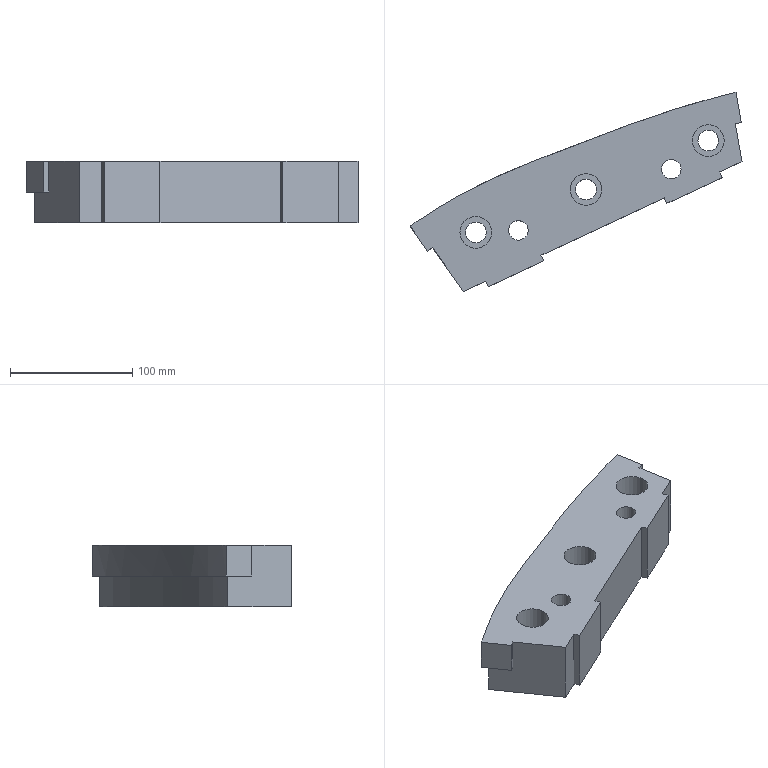Part | NX | features solid 2 | 1 solid | 31 faces | box 271.385 x 162.804 x 50 mm | volume 822513 mm3 | plane 21 | cylinder 8 | spline 2 | commonest cylinder face diameters 17 x3 26 x3 16 x2
STEP:
#1=CARTESIAN_POINT('',(-324.107,502.143,-25.));
#2=VERTEX_POINT('',#1);
#3=CARTESIAN_POINT('',(-319.766,477.523,-25.));
#4=VERTEX_POINT('',#3);
#5=CARTESIAN_POINT('',(-314.512,447.729,-25.));
#6=DIRECTION('',(0.1736,-0.9848,0.));
#7=VECTOR('',#6,1000.);
#8=LINE('',#5,#7);
#9=EDGE_CURVE('',#2,#4,#8,.T.);
#10=ORIENTED_EDGE('',*,*,#9,.T.);
#11=CARTESIAN_POINT('',(-324.69,476.655,-25.));
#12=VERTEX_POINT('',#11);
#13=CARTESIAN_POINT('',(-314.842,478.391,-25.));
#14=DIRECTION('',(-0.9848,-0.1736,0.));
#15=VECTOR('',#14,1000.);
#16=LINE('',#13,#15);
#17=EDGE_CURVE('',#4,#12,#16,.T.);
#18=ORIENTED_EDGE('',*,*,#17,.T.);
#19=CARTESIAN_POINT('',(-328.108,496.039,-25.));
#20=VERTEX_POINT('',#19);
#21=CARTESIAN_POINT('',(-319.436,446.861,-25.));
#22=DIRECTION('',(0.1736,-0.9848,0.));
#23=VECTOR('',#22,1000.);
#24=LINE('',#21,#23);
#25=EDGE_CURVE('',#12,#20,#24,.F.);
#26=ORIENTED_EDGE('',*,*,#25,.T.);
#27=CARTESIAN_POINT('',(-583.566,391.623,-25.));
#28=VERTEX_POINT('',#27);
#29=CARTESIAN_POINT('',(-328.108,496.039,-25.));
#30=CARTESIAN_POINT('',(-339.325,493.302,-25.));
#31=CARTESIAN_POINT('',(-361.624,487.369,-25.));
#32=CARTESIAN_POINT('',(-394.475,476.632,-25.));
#33=CARTESIAN_POINT('',(-427.053,464.52,-25.));
#34=CARTESIAN_POINT('',(-470.494,447.928,-25.));
#35=CARTESIAN_POINT('',(-513.833,431.597,-25.));
#36=CARTESIAN_POINT('',(-554.468,410.285,-25.));
#37=CARTESIAN_POINT('',(-573.98,398.021,-25.));
#38=CARTESIAN_POINT('',(-583.566,391.623,-25.));
#39=B_SPLINE_CURVE_WITH_KNOTS('',3,(#29,#30,#31,#32,#33,#34,#35,#36,#37,#38),.UNSPECIFIED.,.F.,.F.,(4,1,1,1,1,1,1,4),(0.01867,0.1407,0.2627,0.3848,0.5068,0.7508,0.8729,0.9949),.UNSPECIFIED.);
#40=EDGE_CURVE('',#20,#28,#39,.T.);
#41=ORIENTED_EDGE('',*,*,#40,.T.);
#42=CARTESIAN_POINT('',(-572.103,375.253,-25.));
#43=VERTEX_POINT('',#42);
#44=CARTESIAN_POINT('',(-547.462,340.061,-25.));
#45=DIRECTION('',(0.5736,-0.8192,0.));
#46=VECTOR('',#45,1000.);
#47=LINE('',#44,#46);
#48=EDGE_CURVE('',#43,#28,#47,.F.);
#49=ORIENTED_EDGE('',*,*,#48,.F.);
#50=CARTESIAN_POINT('',(-576.199,372.385,-25.));
#51=VERTEX_POINT('',#50);
#52=CARTESIAN_POINT('',(-580.295,369.517,-25.));
#53=DIRECTION('',(0.8192,0.5736,0.));
#54=VECTOR('',#53,1000.);
#55=LINE('',#52,#54);
#56=EDGE_CURVE('',#51,#43,#55,.T.);
#57=ORIENTED_EDGE('',*,*,#56,.F.);
#58=CARTESIAN_POINT('',(-590.588,392.934,-25.));
#59=VERTEX_POINT('',#58);
#60=CARTESIAN_POINT('',(-551.558,337.193,-25.));
#61=DIRECTION('',(0.5736,-0.8192,0.));
#62=VECTOR('',#61,1000.);
#63=LINE('',#60,#62);
#64=EDGE_CURVE('',#59,#51,#63,.T.);
#65=ORIENTED_EDGE('',*,*,#64,.F.);
#66=CARTESIAN_POINT('',(-324.107,502.143,-25.));
#67=CARTESIAN_POINT('',(-341.077,498.12,-25.));
#68=CARTESIAN_POINT('',(-376.687,488.492,-25.));
#69=CARTESIAN_POINT('',(-420.452,472.38,-25.));
#70=CARTESIAN_POINT('',(-456.779,458.517,-25.));
#71=CARTESIAN_POINT('',(-484.05,448.183,-25.));
#72=CARTESIAN_POINT('',(-511.125,437.331,-25.));
#73=CARTESIAN_POINT('',(-546.415,420.942,-25.));
#74=CARTESIAN_POINT('',(-571.409,405.8,-25.));
#75=CARTESIAN_POINT('',(-587.555,394.969,-25.));
#76=CARTESIAN_POINT('',(-595.462,389.665,-25.));
#77=CARTESIAN_POINT('',(-603.368,384.361,-25.));
#78=CARTESIAN_POINT('',(-611.275,379.057,-25.));
#79=B_SPLINE_CURVE_WITH_KNOTS('',3,(#66,#67,#68,#69,#70,#71,#72,#73,#74,#75,#76,#77,#78),.UNSPECIFIED.,.F.,.F.,(4,1,1,1,1,1,1,3,4),(0.,0.1809,0.3825,0.4833,0.5841,0.6849,0.7857,0.9874,1.086),.UNSPECIFIED.);
#80=EDGE_CURVE('',#59,#2,#79,.F.);
#81=ORIENTED_EDGE('',*,*,#80,.T.);
#82=EDGE_LOOP('',(#10,#18,#26,#41,#49,#57,#65,#81));
#83=FACE_BOUND('',#82,.T.);
#84=CARTESIAN_POINT('',(-590.538,392.863,-25.));
#85=DIRECTION('',(0.,0.,-1.));
#86=DIRECTION('',(-1.,0.,0.));
#87=AXIS2_PLACEMENT_3D('',#84,#85,#86);
#88=PLANE('',#87);
#89=ADVANCED_FACE('',(#83),#88,.T.);
#90=CARTESIAN_POINT('',(-368.956,439.339,0.));
#91=VERTEX_POINT('',#90);
#92=CARTESIAN_POINT('',(-376.956,439.339,0.));
#93=DIRECTION('',(0.,0.,1.));
#94=DIRECTION('',(1.,0.,0.));
#95=AXIS2_PLACEMENT_3D('',#92,#93,#94);
#96=CIRCLE('',#95,8.);
#97=EDGE_CURVE('',#91,#91,#96,.T.);
#98=ORIENTED_EDGE('',*,*,#97,.F.);
#99=EDGE_LOOP('',(#98));
#100=FACE_BOUND('',#99,.T.);
#101=CARTESIAN_POINT('',(-493.956,389.339,0.));
#102=VERTEX_POINT('',#101);
#103=CARTESIAN_POINT('',(-501.956,389.339,0.));
#104=DIRECTION('',(0.,0.,1.));
#105=DIRECTION('',(1.,0.,0.));
#106=AXIS2_PLACEMENT_3D('',#103,#104,#105);
#107=CIRCLE('',#106,8.);
#108=EDGE_CURVE('',#102,#102,#107,.T.);
#109=ORIENTED_EDGE('',*,*,#108,.F.);
#110=EDGE_LOOP('',(#109));
#111=FACE_BOUND('',#110,.T.);
#112=CARTESIAN_POINT('',(-459.729,422.741,0.));
#113=VERTEX_POINT('',#112);
#114=CARTESIAN_POINT('',(-446.729,422.741,0.));
#115=DIRECTION('',(0.,0.,-1.));
#116=DIRECTION('',(-1.,0.,0.));
#117=AXIS2_PLACEMENT_3D('',#114,#115,#116);
#118=CIRCLE('',#117,13.);
#119=EDGE_CURVE('',#113,#113,#118,.T.);
#120=ORIENTED_EDGE('',*,*,#119,.T.);
#121=EDGE_LOOP('',(#120));
#122=FACE_BOUND('',#121,.T.);
#123=CARTESIAN_POINT('',(-549.729,387.741,0.));
#124=VERTEX_POINT('',#123);
#125=CARTESIAN_POINT('',(-536.729,387.741,0.));
#126=DIRECTION('',(0.,0.,-1.));
#127=DIRECTION('',(-1.,0.,0.));
#128=AXIS2_PLACEMENT_3D('',#125,#126,#127);
#129=CIRCLE('',#128,13.);
#130=EDGE_CURVE('',#124,#124,#129,.T.);
#131=ORIENTED_EDGE('',*,*,#130,.T.);
#132=EDGE_LOOP('',(#131));
#133=FACE_BOUND('',#132,.T.);
#134=CARTESIAN_POINT('',(-359.729,462.741,0.));
#135=VERTEX_POINT('',#134);
#136=CARTESIAN_POINT('',(-346.729,462.741,0.));
#137=DIRECTION('',(0.,0.,-1.));
#138=DIRECTION('',(-1.,0.,0.));
#139=AXIS2_PLACEMENT_3D('',#136,#137,#138);
#140=CIRCLE('',#139,13.);
#141=EDGE_CURVE('',#135,#135,#140,.T.);
#142=ORIENTED_EDGE('',*,*,#141,.T.);
#143=EDGE_LOOP('',(#142));
#144=FACE_BOUND('',#143,.T.);
#145=CARTESIAN_POINT('',(-319.204,445.542,0.));
#146=VERTEX_POINT('',#145);
#147=CARTESIAN_POINT('',(-324.69,476.655,0.));
#148=VERTEX_POINT('',#147);
#149=CARTESIAN_POINT('',(-319.436,446.861,0.));
#150=DIRECTION('',(-0.1736,0.9848,0.));
#151=VECTOR('',#150,1000.);
#152=LINE('',#149,#151);
#153=EDGE_CURVE('',#146,#148,#152,.T.);
#154=ORIENTED_EDGE('',*,*,#153,.T.);
#155=CARTESIAN_POINT('',(-319.766,477.523,0.));
#156=VERTEX_POINT('',#155);
#157=CARTESIAN_POINT('',(-314.842,478.391,0.));
#158=DIRECTION('',(-0.9848,-0.1736,0.));
#159=VECTOR('',#158,1000.);
#160=LINE('',#157,#159);
#161=EDGE_CURVE('',#156,#148,#160,.T.);
#162=ORIENTED_EDGE('',*,*,#161,.F.);
#163=CARTESIAN_POINT('',(-324.107,502.143,0.));
#164=VERTEX_POINT('',#163);
#165=CARTESIAN_POINT('',(-314.512,447.729,0.));
#166=DIRECTION('',(-0.1736,0.9848,0.));
#167=VECTOR('',#166,1000.);
#168=LINE('',#165,#167);
#169=EDGE_CURVE('',#156,#164,#168,.T.);
#170=ORIENTED_EDGE('',*,*,#169,.T.);
#171=CARTESIAN_POINT('',(-338.626,498.559,0.));
#172=VERTEX_POINT('',#171);
#173=CARTESIAN_POINT('',(-324.107,502.143,0.));
#174=CARTESIAN_POINT('',(-341.077,498.12,0.));
#175=CARTESIAN_POINT('',(-376.687,488.492,0.));
#176=CARTESIAN_POINT('',(-420.452,472.38,0.));
#177=CARTESIAN_POINT('',(-456.779,458.517,0.));
#178=CARTESIAN_POINT('',(-484.05,448.183,0.));
#179=CARTESIAN_POINT('',(-511.125,437.331,0.));
#180=CARTESIAN_POINT('',(-546.415,420.942,0.));
#181=CARTESIAN_POINT('',(-571.409,405.8,0.));
#182=CARTESIAN_POINT('',(-587.555,394.969,0.));
#183=B_SPLINE_CURVE_WITH_KNOTS('',3,(#173,#174,#175,#176,#177,#178,#179,#180,#181,#182),.UNSPECIFIED.,.F.,.F.,(4,1,1,1,1,1,1,4),(0.,0.1809,0.3825,0.4833,0.5841,0.6849,0.7857,0.9874),.UNSPECIFIED.);
#184=EDGE_CURVE('',#164,#172,#183,.T.);
#185=ORIENTED_EDGE('',*,*,#184,.T.);
#186=CARTESIAN_POINT('',(-585.676,396.225,0.));
#187=VERTEX_POINT('',#186);
#188=CARTESIAN_POINT('',(-338.626,498.559,0.));
#189=CARTESIAN_POINT('',(-344.205,497.125,0.));
#190=CARTESIAN_POINT('',(-352.426,494.911,0.));
#191=CARTESIAN_POINT('',(-361.746,492.22,0.));
#192=CARTESIAN_POINT('',(-366.352,490.844,0.));
#193=CARTESIAN_POINT('',(-368.946,490.055,0.));
#194=CARTESIAN_POINT('',(-370.936,489.443,0.));
#195=CARTESIAN_POINT('',(-372.712,488.89,0.));
#196=CARTESIAN_POINT('',(-375.191,488.11,0.));
#197=CARTESIAN_POINT('',(-379.566,486.711,0.));
#198=CARTESIAN_POINT('',(-384.756,485.002,0.));
#199=CARTESIAN_POINT('',(-390.111,483.188,0.));
#200=CARTESIAN_POINT('',(-394.217,481.774,0.));
#201=CARTESIAN_POINT('',(-397.701,480.555,0.));
#202=CARTESIAN_POINT('',(-400.196,479.672,0.));
#203=CARTESIAN_POINT('',(-401.604,479.171,0.));
#204=CARTESIAN_POINT('',(-402.746,478.764,0.));
#205=CARTESIAN_POINT('',(-403.586,478.462,0.));
#206=CARTESIAN_POINT('',(-404.83,478.016,0.));
#207=CARTESIAN_POINT('',(-406.992,477.235,0.));
#208=CARTESIAN_POINT('',(-410.216,476.064,0.));
#209=CARTESIAN_POINT('',(-413.557,474.837,0.));
#210=CARTESIAN_POINT('',(-415.996,473.936,0.));
#211=CARTESIAN_POINT('',(-417.372,473.427,0.));
#212=CARTESIAN_POINT('',(-418.523,472.999,0.));
#213=CARTESIAN_POINT('',(-419.268,472.722,0.));
#214=CARTESIAN_POINT('',(-420.436,472.287,0.));
#215=CARTESIAN_POINT('',(-422.479,471.524,0.));
#216=CARTESIAN_POINT('',(-425.002,470.579,0.));
#217=CARTESIAN_POINT('',(-427.67,469.576,0.));
#218=CARTESIAN_POINT('',(-429.405,468.922,0.));
#219=CARTESIAN_POINT('',(-430.832,468.384,0.));
#220=CARTESIAN_POINT('',(-431.923,467.971,0.));
#221=CARTESIAN_POINT('',(-432.841,467.624,0.));
#222=CARTESIAN_POINT('',(-433.509,467.372,0.));
#223=CARTESIAN_POINT('',(-433.867,467.236,0.));
#224=CARTESIAN_POINT('',(-434.209,467.107,0.));
#225=CARTESIAN_POINT('',(-434.279,467.081,0.));
#226=CARTESIAN_POINT('',(-434.469,467.008,0.));
#227=CARTESIAN_POINT('',(-434.766,466.896,0.));
#228=CARTESIAN_POINT('',(-435.23,466.72,0.));
#229=CARTESIAN_POINT('',(-435.808,466.501,0.));
#230=CARTESIAN_POINT('',(-436.621,466.193,0.));
#231=CARTESIAN_POINT('',(-437.71,465.78,0.));
#232=CARTESIAN_POINT('',(-439.612,465.058,0.));
#233=CARTESIAN_POINT('',(-442.286,464.043,0.));
#234=CARTESIAN_POINT('',(-445.969,462.644,0.));
#235=CARTESIAN_POINT('',(-450.126,461.063,0.));
#236=CARTESIAN_POINT('',(-453.986,459.595,0.));
#237=CARTESIAN_POINT('',(-457.311,458.33,0.));
#238=CARTESIAN_POINT('',(-459.926,457.335,0.));
#239=CARTESIAN_POINT('',(-462.196,456.471,0.));
#240=CARTESIAN_POINT('',(-463.852,455.84,0.));
#241=CARTESIAN_POINT('',(-464.789,455.483,0.));
#242=CARTESIAN_POINT('',(-465.566,455.188,0.));
#243=CARTESIAN_POINT('',(-466.097,454.986,0.));
#244=CARTESIAN_POINT('',(-466.88,454.687,0.));
#245=CARTESIAN_POINT('',(-468.192,454.187,0.));
#246=CARTESIAN_POINT('',(-470.026,453.487,0.));
#247=CARTESIAN_POINT('',(-472.124,452.685,0.));
#248=CARTESIAN_POINT('',(-474.129,451.917,0.));
#249=CARTESIAN_POINT('',(-476.041,451.183,0.));
#250=CARTESIAN_POINT('',(-477.854,450.485,0.));
#251=CARTESIAN_POINT('',(-479.295,449.929,0.));
#252=CARTESIAN_POINT('',(-480.247,449.561,0.));
#253=CARTESIAN_POINT('',(-480.803,449.345,0.));
#254=CARTESIAN_POINT('',(-481.145,449.213,0.));
#255=CARTESIAN_POINT('',(-481.749,448.979,0.));
#256=CARTESIAN_POINT('',(-482.457,448.704,0.));
#257=CARTESIAN_POINT('',(-483.725,448.211,0.));
#258=CARTESIAN_POINT('',(-485.475,447.528,0.));
#259=CARTESIAN_POINT('',(-487.522,446.725,0.));
#260=CARTESIAN_POINT('',(-490.162,445.685,0.));
#261=CARTESIAN_POINT('',(-492.686,444.682,0.));
#262=CARTESIAN_POINT('',(-494.764,443.85,0.));
#263=CARTESIAN_POINT('',(-495.951,443.372,0.));
#264=CARTESIAN_POINT('',(-496.738,443.054,0.));
#265=CARTESIAN_POINT('',(-497.845,442.605,0.));
#266=CARTESIAN_POINT('',(-499.194,442.056,0.));
#267=CARTESIAN_POINT('',(-501.574,441.081,0.));
#268=CARTESIAN_POINT('',(-504.857,439.718,0.));
#269=CARTESIAN_POINT('',(-508.008,438.387,0.));
#270=CARTESIAN_POINT('',(-510.485,437.325,0.));
#271=CARTESIAN_POINT('',(-512.212,436.577,0.));
#272=CARTESIAN_POINT('',(-514.257,435.683,0.));
#273=CARTESIAN_POINT('',(-516.841,434.539,0.));
#274=CARTESIAN_POINT('',(-520.06,433.09,0.));
#275=CARTESIAN_POINT('',(-523.854,431.342,0.));
#276=CARTESIAN_POINT('',(-527.493,429.627,0.));
#277=CARTESIAN_POINT('',(-531.37,427.755,0.));
#278=CARTESIAN_POINT('',(-536.38,425.273,0.));
#279=CARTESIAN_POINT('',(-542.544,422.101,0.));
#280=CARTESIAN_POINT('',(-548.605,418.823,0.));
#281=CARTESIAN_POINT('',(-553.485,416.095,0.));
#282=CARTESIAN_POINT('',(-557.265,413.932,0.));
#283=CARTESIAN_POINT('',(-560.652,411.955,0.));
#284=CARTESIAN_POINT('',(-565.345,409.163,0.));
#285=CARTESIAN_POINT('',(-573.575,404.126,0.));
#286=CARTESIAN_POINT('',(-580.8,399.47,0.));
#287=CARTESIAN_POINT('',(-585.676,396.225,0.));
#288=B_SPLINE_CURVE_WITH_KNOTS('',3,(#188,#189,#190,#191,#192,#193,#194,#195,#196,#197,#198,#199,#200,#201,#202,#203,#204,#205,#206,#207,#208,#209,#210,#211,#212,#213,#214,#215,#216,#217,#218,#219,#220,#221,#222,#223,#224,#225,#226,#227,#228,#229,#230,#231,#232,#233,#234,#235,#236,#237,#238,#239,#240,#241,#242,#243,#244,#245,#246,#247,#248,#249,#250,#251,#252,#253,#254,#255,#256,#257,#258,#259,#260,#261,#262,#263,#264,#265,#266,#267,#268,#269,#270,#271,#272,#273,#274,#275,#276,#277,#278,#279,#280,#281,#282,#283,#284,#285,#286,#287),.UNSPECIFIED.,.F.,.F.,(4,1,1,1,1,1,1,1,1,1,1,1,1,1,1,1,1,1,1,1,1,1,1,1,1,1,1,1,1,1,1,1,1,1,1,1,1,1,1,1,1,1,1,1,1,1,1,1,1,1,1,1,1,1,1,1,1,1,1,1,1,1,1,1,1,1,1,1,1,1,1,1,1,1,1,1,1,1,1,1,1,1,1,1,1,1,1,1,1,1,1,1,1,1,1,1,1,4),(0.,0.0625,0.09375,0.1094,0.1172,0.125,0.1328,0.1406,0.1562,0.1875,0.2031,0.2188,0.2344,0.2422,0.2461,0.25,0.2539,0.2578,0.2656,0.2812,0.2969,0.3047,0.3086,0.3125,0.3164,0.3203,0.3281,0.3438,0.3516,0.3594,0.3633,0.3672,0.3711,0.373,0.374,0.375,0.376,0.377,0.3789,0.3828,0.3867,0.3906,0.3984,0.4062,0.4219,0.4375,0.4531,0.4688,0.4766,0.4844,0.4922,0.4961,0.498,0.5,0.502,0.5039,0.5078,0.5156,0.5234,0.5312,0.5391,0.5469,0.5547,0.5586,0.5605,0.5625,0.5645,0.5664,0.5703,0.5781,0.5859,0.5938,0.6094,0.6172,0.6211,0.625,0.6289,0.6328,0.6406,0.6562,0.6719,0.6797,0.6875,0.6953,0.7031,0.7188,0.7344,0.75,0.7656,0.7812,0.8125,0.8438,0.8594,0.875,0.8906,0.9062,0.9375,1.),.UNSPECIFIED.);
#289=EDGE_CURVE('',#172,#187,#288,.T.);
#290=ORIENTED_EDGE('',*,*,#289,.T.);
#291=CARTESIAN_POINT('',(-587.555,394.969,0.));
#292=VERTEX_POINT('',#291);
#293=CARTESIAN_POINT('',(-324.107,502.143,0.));
#294=CARTESIAN_POINT('',(-341.077,498.12,0.));
#295=CARTESIAN_POINT('',(-376.687,488.492,0.));
#296=CARTESIAN_POINT('',(-420.452,472.38,0.));
#297=CARTESIAN_POINT('',(-456.779,458.517,0.));
#298=CARTESIAN_POINT('',(-484.05,448.183,0.));
#299=CARTESIAN_POINT('',(-511.125,437.331,0.));
#300=CARTESIAN_POINT('',(-546.415,420.942,0.));
#301=CARTESIAN_POINT('',(-571.409,405.8,0.));
#302=CARTESIAN_POINT('',(-587.555,394.969,0.));
#303=B_SPLINE_CURVE_WITH_KNOTS('',3,(#293,#294,#295,#296,#297,#298,#299,#300,#301,#302),.UNSPECIFIED.,.F.,.F.,(4,1,1,1,1,1,1,4),(0.,0.1809,0.3825,0.4833,0.5841,0.6849,0.7857,0.9874),.UNSPECIFIED.);
#304=EDGE_CURVE('',#187,#292,#303,.T.);
#305=ORIENTED_EDGE('',*,*,#304,.T.);
#306=CARTESIAN_POINT('',(-590.588,392.934,0.));
#307=VERTEX_POINT('',#306);
#308=CARTESIAN_POINT('',(-587.555,394.969,0.));
#309=CARTESIAN_POINT('',(-588.566,394.291,0.));
#310=CARTESIAN_POINT('',(-589.577,393.613,0.));
#311=CARTESIAN_POINT('',(-590.588,392.934,0.));
#312=B_SPLINE_CURVE_WITH_KNOTS('',3,(#308,#309,#310,#311),.UNSPECIFIED.,.F.,.F.,(4,4),(0.,0.003652),.UNSPECIFIED.);
#313=EDGE_CURVE('',#292,#307,#312,.T.);
#314=ORIENTED_EDGE('',*,*,#313,.T.);
#315=CARTESIAN_POINT('',(-576.199,372.385,0.));
#316=VERTEX_POINT('',#315);
#317=CARTESIAN_POINT('',(-551.558,337.193,0.));
#318=DIRECTION('',(-0.5736,0.8192,0.));
#319=VECTOR('',#318,1000.);
#320=LINE('',#317,#319);
#321=EDGE_CURVE('',#316,#307,#320,.T.);
#322=ORIENTED_EDGE('',*,*,#321,.F.);
#323=CARTESIAN_POINT('',(-572.103,375.253,0.));
#324=VERTEX_POINT('',#323);
#325=CARTESIAN_POINT('',(-580.295,369.517,0.));
#326=DIRECTION('',(0.8192,0.5736,0.));
#327=VECTOR('',#326,1000.);
#328=LINE('',#325,#327);
#329=EDGE_CURVE('',#316,#324,#328,.T.);
#330=ORIENTED_EDGE('',*,*,#329,.T.);
#331=CARTESIAN_POINT('',(-546.956,339.339,0.));
#332=VERTEX_POINT('',#331);
#333=CARTESIAN_POINT('',(-547.462,340.061,0.));
#334=DIRECTION('',(-0.5736,0.8192,0.));
#335=VECTOR('',#334,1000.);
#336=LINE('',#333,#335);
#337=EDGE_CURVE('',#332,#324,#336,.T.);
#338=ORIENTED_EDGE('',*,*,#337,.F.);
#339=CARTESIAN_POINT('',(-528.83,347.791,0.));
#340=VERTEX_POINT('',#339);
#341=CARTESIAN_POINT('',(-551.558,337.193,0.));
#342=DIRECTION('',(0.9063,0.4226,0.));
#343=VECTOR('',#342,1000.);
#344=LINE('',#341,#343);
#345=EDGE_CURVE('',#332,#340,#344,.T.);
#346=ORIENTED_EDGE('',*,*,#345,.T.);
#347=CARTESIAN_POINT('',(-526.717,343.26,0.));
#348=VERTEX_POINT('',#347);
#349=CARTESIAN_POINT('',(-528.83,347.791,0.));
#350=DIRECTION('',(-0.4226,0.9063,0.));
#351=VECTOR('',#350,1000.);
#352=LINE('',#349,#351);
#353=EDGE_CURVE('',#340,#348,#352,.F.);
#354=ORIENTED_EDGE('',*,*,#353,.T.);
#355=CARTESIAN_POINT('',(-481.402,364.391,0.));
#356=VERTEX_POINT('',#355);
#357=CARTESIAN_POINT('',(-549.445,332.662,0.));
#358=DIRECTION('',(0.9063,0.4226,0.));
#359=VECTOR('',#358,1000.);
#360=LINE('',#357,#359);
#361=EDGE_CURVE('',#348,#356,#360,.T.);
#362=ORIENTED_EDGE('',*,*,#361,.T.);
#363=CARTESIAN_POINT('',(-483.515,368.922,0.));
#364=VERTEX_POINT('',#363);
#365=CARTESIAN_POINT('',(-483.515,368.922,0.));
#366=DIRECTION('',(0.4226,-0.9063,0.));
#367=VECTOR('',#366,1000.);
#368=LINE('',#365,#367);
#369=EDGE_CURVE('',#364,#356,#368,.T.);
#370=ORIENTED_EDGE('',*,*,#369,.F.);
#371=CARTESIAN_POINT('',(-382.645,415.958,0.));
#372=VERTEX_POINT('',#371);
#373=CARTESIAN_POINT('',(-551.558,337.193,0.));
#374=DIRECTION('',(0.9063,0.4226,0.));
#375=VECTOR('',#374,1000.);
#376=LINE('',#373,#375);
#377=EDGE_CURVE('',#364,#372,#376,.T.);
#378=ORIENTED_EDGE('',*,*,#377,.T.);
#379=CARTESIAN_POINT('',(-380.532,411.427,0.));
#380=VERTEX_POINT('',#379);
#381=CARTESIAN_POINT('',(-382.645,415.958,0.));
#382=DIRECTION('',(-0.4226,0.9063,0.));
#383=VECTOR('',#382,1000.);
#384=LINE('',#381,#383);
#385=EDGE_CURVE('',#372,#380,#384,.F.);
#386=ORIENTED_EDGE('',*,*,#385,.T.);
#387=CARTESIAN_POINT('',(-335.217,432.558,0.));
#388=VERTEX_POINT('',#387);
#389=CARTESIAN_POINT('',(-385.133,409.281,0.));
#390=DIRECTION('',(0.9063,0.4226,0.));
#391=VECTOR('',#390,1000.);
#392=LINE('',#389,#391);
#393=EDGE_CURVE('',#380,#388,#392,.T.);
#394=ORIENTED_EDGE('',*,*,#393,.T.);
#395=CARTESIAN_POINT('',(-337.33,437.089,0.));
#396=VERTEX_POINT('',#395);
#397=CARTESIAN_POINT('',(-337.33,437.089,0.));
#398=DIRECTION('',(0.4226,-0.9063,0.));
#399=VECTOR('',#398,1000.);
#400=LINE('',#397,#399);
#401=EDGE_CURVE('',#396,#388,#400,.T.);
#402=ORIENTED_EDGE('',*,*,#401,.F.);
#403=CARTESIAN_POINT('',(-551.558,337.193,0.));
#404=DIRECTION('',(0.9063,0.4226,0.));
#405=VECTOR('',#404,1000.);
#406=LINE('',#403,#405);
#407=EDGE_CURVE('',#396,#146,#406,.T.);
#408=ORIENTED_EDGE('',*,*,#407,.T.);
#409=EDGE_LOOP('',(#154,#162,#170,#185,#290,#305,#314,#322,#330,#338,#346,#354,#362,#370,#378,#386,#394,#402,#408));
#410=FACE_BOUND('',#409,.T.);
#411=CARTESIAN_POINT('',(-524.47,294.913,0.));
#412=DIRECTION('',(0.,0.,1.));
#413=DIRECTION('',(1.,0.,0.));
#414=AXIS2_PLACEMENT_3D('',#411,#412,#413);
#415=PLANE('',#414);
#416=ADVANCED_FACE('',(#100,#111,#122,#133,#144,#410),#415,.T.);
#417=ORIENTED_EDGE('',*,*,#169,.F.);
#418=CARTESIAN_POINT('',(-319.766,477.523,-50.));
#419=DIRECTION('',(0.,0.,-1.));
#420=VECTOR('',#419,1000.);
#421=LINE('',#418,#420);
#422=EDGE_CURVE('',#156,#4,#421,.T.);
#423=ORIENTED_EDGE('',*,*,#422,.T.);
#424=ORIENTED_EDGE('',*,*,#9,.F.);
#425=CARTESIAN_POINT('',(-324.107,502.143,-50.));
#426=DIRECTION('',(0.,0.,1.));
#427=VECTOR('',#426,1000.);
#428=LINE('',#425,#427);
#429=EDGE_CURVE('',#2,#164,#428,.T.);
#430=ORIENTED_EDGE('',*,*,#429,.T.);
#431=EDGE_LOOP('',(#417,#423,#424,#430));
#432=FACE_BOUND('',#431,.T.);
#433=CARTESIAN_POINT('',(-314.512,447.729,-50.));
#434=DIRECTION('',(0.9848,0.1736,0.));
#435=DIRECTION('',(-0.1736,0.9848,0.));
#436=AXIS2_PLACEMENT_3D('',#433,#434,#435);
#437=PLANE('',#436);
#438=ADVANCED_FACE('',(#432),#437,.T.);
#439=CARTESIAN_POINT('',(-319.204,445.542,-50.));
#440=VERTEX_POINT('',#439);
#441=CARTESIAN_POINT('',(-319.204,445.542,-50.));
#442=DIRECTION('',(0.,0.,-1.));
#443=VECTOR('',#442,1000.);
#444=LINE('',#441,#443);
#445=EDGE_CURVE('',#146,#440,#444,.T.);
#446=ORIENTED_EDGE('',*,*,#445,.F.);
#447=ORIENTED_EDGE('',*,*,#407,.F.);
#448=CARTESIAN_POINT('',(-337.33,437.089,-50.));
#449=VERTEX_POINT('',#448);
#450=CARTESIAN_POINT('',(-337.33,437.089,-50.));
#451=DIRECTION('',(0.,0.,-1.));
#452=VECTOR('',#451,1000.);
#453=LINE('',#450,#452);
#454=EDGE_CURVE('',#396,#449,#453,.T.);
#455=ORIENTED_EDGE('',*,*,#454,.T.);
#456=CARTESIAN_POINT('',(-551.558,337.193,-50.));
#457=DIRECTION('',(0.9063,0.4226,0.));
#458=VECTOR('',#457,1000.);
#459=LINE('',#456,#458);
#460=EDGE_CURVE('',#449,#440,#459,.T.);
#461=ORIENTED_EDGE('',*,*,#460,.T.);
#462=EDGE_LOOP('',(#446,#447,#455,#461));
#463=FACE_BOUND('',#462,.T.);
#464=CARTESIAN_POINT('',(-551.558,337.193,-50.));
#465=DIRECTION('',(0.4226,-0.9063,0.));
#466=DIRECTION('',(0.9063,0.4226,0.));
#467=AXIS2_PLACEMENT_3D('',#464,#465,#466);
#468=PLANE('',#467);
#469=ADVANCED_FACE('',(#463),#468,.T.);
#470=CARTESIAN_POINT('',(-455.229,422.741,-25.));
#471=VERTEX_POINT('',#470);
#472=CARTESIAN_POINT('',(-446.729,422.741,-25.));
#473=DIRECTION('',(0.,0.,-1.));
#474=DIRECTION('',(-1.,0.,0.));
#475=AXIS2_PLACEMENT_3D('',#472,#473,#474);
#476=CIRCLE('',#475,8.5);
#477=EDGE_CURVE('',#471,#471,#476,.F.);
#478=ORIENTED_EDGE('',*,*,#477,.T.);
#479=EDGE_LOOP('',(#478));
#480=FACE_BOUND('',#479,.T.);
#481=CARTESIAN_POINT('',(-455.229,422.741,-50.));
#482=VERTEX_POINT('',#481);
#483=CARTESIAN_POINT('',(-446.729,422.741,-50.));
#484=DIRECTION('',(0.,0.,-1.));
#485=DIRECTION('',(-1.,0.,0.));
#486=AXIS2_PLACEMENT_3D('',#483,#484,#485);
#487=CIRCLE('',#486,8.5);
#488=EDGE_CURVE('',#482,#482,#487,.T.);
#489=ORIENTED_EDGE('',*,*,#488,.T.);
#490=EDGE_LOOP('',(#489));
#491=FACE_BOUND('',#490,.T.);
#492=CARTESIAN_POINT('',(-446.729,422.741,-75.));
#493=DIRECTION('',(0.,0.,1.));
#494=DIRECTION('',(1.,0.,0.));
#495=AXIS2_PLACEMENT_3D('',#492,#493,#494);
#496=CYLINDRICAL_SURFACE('',#495,8.5);
#497=ADVANCED_FACE('',(#480,#491),#496,.F.);
#498=ORIENTED_EDGE('',*,*,#477,.F.);
#499=EDGE_LOOP('',(#498));
#500=FACE_BOUND('',#499,.T.);
#501=CARTESIAN_POINT('',(-433.729,422.741,-25.));
#502=VERTEX_POINT('',#501);
#503=CARTESIAN_POINT('',(-446.729,422.741,-25.));
#504=DIRECTION('',(0.,0.,1.));
#505=DIRECTION('',(1.,0.,0.));
#506=AXIS2_PLACEMENT_3D('',#503,#504,#505);
#507=CIRCLE('',#506,13.);
#508=EDGE_CURVE('',#502,#502,#507,.T.);
#509=ORIENTED_EDGE('',*,*,#508,.T.);
#510=EDGE_LOOP('',(#509));
#511=FACE_BOUND('',#510,.T.);
#512=CARTESIAN_POINT('',(-446.729,422.741,-25.));
#513=DIRECTION('',(0.,0.,-1.));
#514=DIRECTION('',(-1.,0.,0.));
#515=AXIS2_PLACEMENT_3D('',#512,#513,#514);
#516=PLANE('',#515);
#517=ADVANCED_FACE('',(#500,#511),#516,.F.);
#518=ORIENTED_EDGE('',*,*,#119,.F.);
#519=EDGE_LOOP('',(#518));
#520=FACE_BOUND('',#519,.T.);
#521=ORIENTED_EDGE('',*,*,#508,.F.);
#522=EDGE_LOOP('',(#521));
#523=FACE_BOUND('',#522,.T.);
#524=CARTESIAN_POINT('',(-446.729,422.741,-25.));
#525=DIRECTION('',(0.,0.,1.));
#526=DIRECTION('',(1.,0.,0.));
#527=AXIS2_PLACEMENT_3D('',#524,#525,#526);
#528=CYLINDRICAL_SURFACE('',#527,13.);
#529=ADVANCED_FACE('',(#520,#523),#528,.F.);
#530=CARTESIAN_POINT('',(-368.956,439.339,-50.));
#531=VERTEX_POINT('',#530);
#532=CARTESIAN_POINT('',(-376.956,439.339,-50.));
#533=DIRECTION('',(0.,0.,1.));
#534=DIRECTION('',(1.,0.,0.));
#535=AXIS2_PLACEMENT_3D('',#532,#533,#534);
#536=CIRCLE('',#535,8.);
#537=EDGE_CURVE('',#531,#531,#536,.T.);
#538=ORIENTED_EDGE('',*,*,#537,.T.);
#539=EDGE_LOOP('',(#538));
#540=FACE_BOUND('',#539,.T.);
#541=CARTESIAN_POINT('',(-493.956,389.339,-50.));
#542=VERTEX_POINT('',#541);
#543=CARTESIAN_POINT('',(-501.956,389.339,-50.));
#544=DIRECTION('',(0.,0.,1.));
#545=DIRECTION('',(1.,0.,0.));
#546=AXIS2_PLACEMENT_3D('',#543,#544,#545);
#547=CIRCLE('',#546,8.);
#548=EDGE_CURVE('',#542,#542,#547,.T.);
#549=ORIENTED_EDGE('',*,*,#548,.T.);
#550=EDGE_LOOP('',(#549));
#551=FACE_BOUND('',#550,.T.);
#552=CARTESIAN_POINT('',(-328.108,496.039,-50.));
#553=VERTEX_POINT('',#552);
#554=CARTESIAN_POINT('',(-582.88,392.08,-50.));
#555=VERTEX_POINT('',#554);
#556=CARTESIAN_POINT('',(-328.108,496.039,-50.));
#557=CARTESIAN_POINT('',(-339.298,493.309,-50.));
#558=CARTESIAN_POINT('',(-361.545,487.392,-50.));
#559=CARTESIAN_POINT('',(-394.405,476.656,-50.));
#560=CARTESIAN_POINT('',(-426.816,464.611,-50.));
#561=CARTESIAN_POINT('',(-469.87,448.16,-50.));
#562=CARTESIAN_POINT('',(-513.032,431.936,-50.));
#563=CARTESIAN_POINT('',(-553.719,410.721,-50.));
#564=CARTESIAN_POINT('',(-573.255,398.485,-50.));
#565=CARTESIAN_POINT('',(-582.88,392.08,-50.));
#566=B_SPLINE_CURVE_WITH_KNOTS('',3,(#556,#557,#558,#559,#560,#561,#562,#563,#564,#565),.UNSPECIFIED.,.F.,.F.,(4,1,1,1,1,1,1,4),(0.01029,0.04482,0.07935,0.1139,0.1484,0.2175,0.252,0.2865),.UNSPECIFIED.);
#567=EDGE_CURVE('',#553,#555,#566,.T.);
#568=ORIENTED_EDGE('',*,*,#567,.F.);
#569=CARTESIAN_POINT('',(-325.475,481.108,-50.));
#570=DIRECTION('',(-0.1736,0.9848,0.));
#571=VECTOR('',#570,1000.);
#572=LINE('',#569,#571);
#573=EDGE_CURVE('',#440,#553,#572,.T.);
#574=ORIENTED_EDGE('',*,*,#573,.F.);
#575=ORIENTED_EDGE('',*,*,#460,.F.);
#576=CARTESIAN_POINT('',(-335.217,432.558,-50.));
#577=VERTEX_POINT('',#576);
#578=CARTESIAN_POINT('',(-337.33,437.089,-50.));
#579=DIRECTION('',(0.4226,-0.9063,0.));
#580=VECTOR('',#579,1000.);
#581=LINE('',#578,#580);
#582=EDGE_CURVE('',#449,#577,#581,.T.);
#583=ORIENTED_EDGE('',*,*,#582,.T.);
#584=CARTESIAN_POINT('',(-380.532,411.427,-50.));
#585=VERTEX_POINT('',#584);
#586=CARTESIAN_POINT('',(-385.133,409.281,-50.));
#587=DIRECTION('',(0.9063,0.4226,0.));
#588=VECTOR('',#587,1000.);
#589=LINE('',#586,#588);
#590=EDGE_CURVE('',#585,#577,#589,.T.);
#591=ORIENTED_EDGE('',*,*,#590,.F.);
#592=CARTESIAN_POINT('',(-382.645,415.958,-50.));
#593=VERTEX_POINT('',#592);
#594=CARTESIAN_POINT('',(-382.645,415.958,-50.));
#595=DIRECTION('',(-0.4226,0.9063,0.));
#596=VECTOR('',#595,1000.);
#597=LINE('',#594,#596);
#598=EDGE_CURVE('',#593,#585,#597,.F.);
#599=ORIENTED_EDGE('',*,*,#598,.F.);
#600=CARTESIAN_POINT('',(-483.515,368.922,-50.));
#601=VERTEX_POINT('',#600);
#602=CARTESIAN_POINT('',(-551.558,337.193,-50.));
#603=DIRECTION('',(0.9063,0.4226,0.));
#604=VECTOR('',#603,1000.);
#605=LINE('',#602,#604);
#606=EDGE_CURVE('',#601,#593,#605,.T.);
#607=ORIENTED_EDGE('',*,*,#606,.F.);
#608=CARTESIAN_POINT('',(-481.402,364.391,-50.));
#609=VERTEX_POINT('',#608);
#610=CARTESIAN_POINT('',(-483.515,368.922,-50.));
#611=DIRECTION('',(0.4226,-0.9063,0.));
#612=VECTOR('',#611,1000.);
#613=LINE('',#610,#612);
#614=EDGE_CURVE('',#601,#609,#613,.T.);
#615=ORIENTED_EDGE('',*,*,#614,.T.);
#616=CARTESIAN_POINT('',(-526.717,343.26,-50.));
#617=VERTEX_POINT('',#616);
#618=CARTESIAN_POINT('',(-549.445,332.662,-50.));
#619=DIRECTION('',(0.9063,0.4226,0.));
#620=VECTOR('',#619,1000.);
#621=LINE('',#618,#620);
#622=EDGE_CURVE('',#617,#609,#621,.T.);
#623=ORIENTED_EDGE('',*,*,#622,.F.);
#624=CARTESIAN_POINT('',(-528.83,347.791,-50.));
#625=VERTEX_POINT('',#624);
#626=CARTESIAN_POINT('',(-528.83,347.791,-50.));
#627=DIRECTION('',(-0.4226,0.9063,0.));
#628=VECTOR('',#627,1000.);
#629=LINE('',#626,#628);
#630=EDGE_CURVE('',#625,#617,#629,.F.);
#631=ORIENTED_EDGE('',*,*,#630,.F.);
#632=CARTESIAN_POINT('',(-546.956,339.339,-50.));
#633=VERTEX_POINT('',#632);
#634=CARTESIAN_POINT('',(-551.558,337.193,-50.));
#635=DIRECTION('',(0.9063,0.4226,0.));
#636=VECTOR('',#635,1000.);
#637=LINE('',#634,#636);
#638=EDGE_CURVE('',#633,#625,#637,.T.);
#639=ORIENTED_EDGE('',*,*,#638,.F.);
#640=CARTESIAN_POINT('',(-583.56,391.614,-50.));
#641=VERTEX_POINT('',#640);
#642=CARTESIAN_POINT('',(-573.713,377.551,-50.));
#643=DIRECTION('',(-0.5736,0.8192,0.));
#644=VECTOR('',#643,1000.);
#645=LINE('',#642,#644);
#646=EDGE_CURVE('',#633,#641,#645,.T.);
#647=ORIENTED_EDGE('',*,*,#646,.T.);
#648=CARTESIAN_POINT('',(-583.56,391.614,-50.));
#649=CARTESIAN_POINT('',(-583.333,391.769,-50.));
#650=CARTESIAN_POINT('',(-583.107,391.924,-50.));
#651=CARTESIAN_POINT('',(-582.88,392.08,-50.));
#652=B_SPLINE_CURVE_WITH_KNOTS('',3,(#648,#649,#650,#651),.UNSPECIFIED.,.F.,.F.,(4,4),(0.0003381,0.003542),.UNSPECIFIED.);
#653=EDGE_CURVE('',#555,#641,#652,.F.);
#654=ORIENTED_EDGE('',*,*,#653,.F.);
#655=EDGE_LOOP('',(#568,#574,#575,#583,#591,#599,#607,#615,#623,#631,#639,#647,#654));
#656=FACE_BOUND('',#655,.T.);
#657=CARTESIAN_POINT('',(-545.229,387.741,-50.));
#658=VERTEX_POINT('',#657);
#659=CARTESIAN_POINT('',(-536.729,387.741,-50.));
#660=DIRECTION('',(0.,0.,-1.));
#661=DIRECTION('',(-1.,0.,0.));
#662=AXIS2_PLACEMENT_3D('',#659,#660,#661);
#663=CIRCLE('',#662,8.5);
#664=EDGE_CURVE('',#658,#658,#663,.T.);
#665=ORIENTED_EDGE('',*,*,#664,.F.);
#666=EDGE_LOOP('',(#665));
#667=FACE_BOUND('',#666,.T.);
#668=CARTESIAN_POINT('',(-355.229,462.741,-50.));
#669=VERTEX_POINT('',#668);
#670=CARTESIAN_POINT('',(-346.729,462.741,-50.));
#671=DIRECTION('',(0.,0.,-1.));
#672=DIRECTION('',(-1.,0.,0.));
#673=AXIS2_PLACEMENT_3D('',#670,#671,#672);
#674=CIRCLE('',#673,8.5);
#675=EDGE_CURVE('',#669,#669,#674,.T.);
#676=ORIENTED_EDGE('',*,*,#675,.F.);
#677=EDGE_LOOP('',(#676));
#678=FACE_BOUND('',#677,.T.);
#679=ORIENTED_EDGE('',*,*,#488,.F.);
#680=EDGE_LOOP('',(#679));
#681=FACE_BOUND('',#680,.T.);
#682=CARTESIAN_POINT('',(-59.718,-803.606,-50.));
#683=DIRECTION('',(0.,0.,1.));
#684=DIRECTION('',(1.,0.,0.));
#685=AXIS2_PLACEMENT_3D('',#682,#683,#684);
#686=PLANE('',#685);
#687=ADVANCED_FACE('',(#540,#551,#656,#667,#678,#681),#686,.F.);
#688=CARTESIAN_POINT('',(-523.729,387.741,-25.));
#689=VERTEX_POINT('',#688);
#690=CARTESIAN_POINT('',(-536.729,387.741,-25.));
#691=DIRECTION('',(0.,0.,1.));
#692=DIRECTION('',(1.,0.,0.));
#693=AXIS2_PLACEMENT_3D('',#690,#691,#692);
#694=CIRCLE('',#693,13.);
#695=EDGE_CURVE('',#689,#689,#694,.T.);
#696=ORIENTED_EDGE('',*,*,#695,.T.);
#697=EDGE_LOOP('',(#696));
#698=FACE_BOUND('',#697,.T.);
#699=CARTESIAN_POINT('',(-545.229,387.741,-25.));
#700=VERTEX_POINT('',#699);
#701=CARTESIAN_POINT('',(-536.729,387.741,-25.));
#702=DIRECTION('',(0.,0.,-1.));
#703=DIRECTION('',(-1.,0.,0.));
#704=AXIS2_PLACEMENT_3D('',#701,#702,#703);
#705=CIRCLE('',#704,8.5);
#706=EDGE_CURVE('',#700,#700,#705,.F.);
#707=ORIENTED_EDGE('',*,*,#706,.F.);
#708=EDGE_LOOP('',(#707));
#709=FACE_BOUND('',#708,.T.);
#710=CARTESIAN_POINT('',(-536.729,387.741,-25.));
#711=DIRECTION('',(0.,0.,-1.));
#712=DIRECTION('',(-1.,0.,0.));
#713=AXIS2_PLACEMENT_3D('',#710,#711,#712);
#714=PLANE('',#713);
#715=ADVANCED_FACE('',(#698,#709),#714,.F.);
#716=ORIENTED_EDGE('',*,*,#664,.T.);
#717=EDGE_LOOP('',(#716));
#718=FACE_BOUND('',#717,.T.);
#719=ORIENTED_EDGE('',*,*,#706,.T.);
#720=EDGE_LOOP('',(#719));
#721=FACE_BOUND('',#720,.T.);
#722=CARTESIAN_POINT('',(-536.729,387.741,-75.));
#723=DIRECTION('',(0.,0.,1.));
#724=DIRECTION('',(1.,0.,0.));
#725=AXIS2_PLACEMENT_3D('',#722,#723,#724);
#726=CYLINDRICAL_SURFACE('',#725,8.5);
#727=ADVANCED_FACE('',(#718,#721),#726,.F.);
#728=ORIENTED_EDGE('',*,*,#130,.F.);
#729=EDGE_LOOP('',(#728));
#730=FACE_BOUND('',#729,.T.);
#731=ORIENTED_EDGE('',*,*,#695,.F.);
#732=EDGE_LOOP('',(#731));
#733=FACE_BOUND('',#732,.T.);
#734=CARTESIAN_POINT('',(-536.729,387.741,-25.));
#735=DIRECTION('',(0.,0.,1.));
#736=DIRECTION('',(1.,0.,0.));
#737=AXIS2_PLACEMENT_3D('',#734,#735,#736);
#738=CYLINDRICAL_SURFACE('',#737,13.);
#739=ADVANCED_FACE('',(#730,#733),#738,.F.);
#740=CARTESIAN_POINT('',(-355.229,462.741,-25.));
#741=VERTEX_POINT('',#740);
#742=CARTESIAN_POINT('',(-346.729,462.741,-25.));
#743=DIRECTION('',(0.,0.,-1.));
#744=DIRECTION('',(-1.,0.,0.));
#745=AXIS2_PLACEMENT_3D('',#742,#743,#744);
#746=CIRCLE('',#745,8.5);
#747=EDGE_CURVE('',#741,#741,#746,.F.);
#748=ORIENTED_EDGE('',*,*,#747,.F.);
#749=EDGE_LOOP('',(#748));
#750=FACE_BOUND('',#749,.T.);
#751=CARTESIAN_POINT('',(-333.729,462.741,-25.));
#752=VERTEX_POINT('',#751);
#753=CARTESIAN_POINT('',(-346.729,462.741,-25.));
#754=DIRECTION('',(0.,0.,1.));
#755=DIRECTION('',(1.,0.,0.));
#756=AXIS2_PLACEMENT_3D('',#753,#754,#755);
#757=CIRCLE('',#756,13.);
#758=EDGE_CURVE('',#752,#752,#757,.T.);
#759=ORIENTED_EDGE('',*,*,#758,.T.);
#760=EDGE_LOOP('',(#759));
#761=FACE_BOUND('',#760,.T.);
#762=CARTESIAN_POINT('',(-346.729,462.741,-25.));
#763=DIRECTION('',(0.,0.,-1.));
#764=DIRECTION('',(-1.,0.,0.));
#765=AXIS2_PLACEMENT_3D('',#762,#763,#764);
#766=PLANE('',#765);
#767=ADVANCED_FACE('',(#750,#761),#766,.F.);
#768=ORIENTED_EDGE('',*,*,#675,.T.);
#769=EDGE_LOOP('',(#768));
#770=FACE_BOUND('',#769,.T.);
#771=ORIENTED_EDGE('',*,*,#747,.T.);
#772=EDGE_LOOP('',(#771));
#773=FACE_BOUND('',#772,.T.);
#774=CARTESIAN_POINT('',(-346.729,462.741,-75.));
#775=DIRECTION('',(0.,0.,1.));
#776=DIRECTION('',(1.,0.,0.));
#777=AXIS2_PLACEMENT_3D('',#774,#775,#776);
#778=CYLINDRICAL_SURFACE('',#777,8.5);
#779=ADVANCED_FACE('',(#770,#773),#778,.F.);
#780=ORIENTED_EDGE('',*,*,#141,.F.);
#781=EDGE_LOOP('',(#780));
#782=FACE_BOUND('',#781,.T.);
#783=ORIENTED_EDGE('',*,*,#758,.F.);
#784=EDGE_LOOP('',(#783));
#785=FACE_BOUND('',#784,.T.);
#786=CARTESIAN_POINT('',(-346.729,462.741,-25.));
#787=DIRECTION('',(0.,0.,1.));
#788=DIRECTION('',(1.,0.,0.));
#789=AXIS2_PLACEMENT_3D('',#786,#787,#788);
#790=CYLINDRICAL_SURFACE('',#789,13.);
#791=ADVANCED_FACE('',(#782,#785),#790,.F.);
#792=ORIENTED_EDGE('',*,*,#598,.T.);
#793=CARTESIAN_POINT('',(-380.532,411.427,-50.));
#794=DIRECTION('',(0.,0.,-1.));
#795=VECTOR('',#794,1000.);
#796=LINE('',#793,#795);
#797=EDGE_CURVE('',#585,#380,#796,.F.);
#798=ORIENTED_EDGE('',*,*,#797,.T.);
#799=ORIENTED_EDGE('',*,*,#385,.F.);
#800=CARTESIAN_POINT('',(-382.645,415.958,-50.));
#801=DIRECTION('',(0.,0.,1.));
#802=VECTOR('',#801,1000.);
#803=LINE('',#800,#802);
#804=EDGE_CURVE('',#372,#593,#803,.F.);
#805=ORIENTED_EDGE('',*,*,#804,.T.);
#806=EDGE_LOOP('',(#792,#798,#799,#805));
#807=FACE_BOUND('',#806,.T.);
#808=CARTESIAN_POINT('',(-382.645,415.958,-50.));
#809=DIRECTION('',(-0.9063,-0.4226,0.));
#810=DIRECTION('',(0.4226,-0.9063,0.));
#811=AXIS2_PLACEMENT_3D('',#808,#809,#810);
#812=PLANE('',#811);
#813=ADVANCED_FACE('',(#807),#812,.T.);
#814=ORIENTED_EDGE('',*,*,#64,.T.);
#815=CARTESIAN_POINT('',(-576.199,372.385,-50.));
#816=DIRECTION('',(0.,0.,1.));
#817=VECTOR('',#816,1000.);
#818=LINE('',#815,#817);
#819=EDGE_CURVE('',#51,#316,#818,.T.);
#820=ORIENTED_EDGE('',*,*,#819,.T.);
#821=ORIENTED_EDGE('',*,*,#321,.T.);
#822=CARTESIAN_POINT('',(-590.588,392.934,-25.));
#823=DIRECTION('',(0.,0.,1.));
#824=VECTOR('',#823,1000.);
#825=LINE('',#822,#824);
#826=EDGE_CURVE('',#59,#307,#825,.T.);
#827=ORIENTED_EDGE('',*,*,#826,.F.);
#828=EDGE_LOOP('',(#814,#820,#821,#827));
#829=FACE_BOUND('',#828,.T.);
#830=CARTESIAN_POINT('',(-551.558,337.193,-50.));
#831=DIRECTION('',(0.8192,0.5736,0.));
#832=DIRECTION('',(-0.5736,0.8192,0.));
#833=AXIS2_PLACEMENT_3D('',#830,#831,#832);
#834=PLANE('',#833);
#835=ADVANCED_FACE('',(#829),#834,.F.);
#836=ORIENTED_EDGE('',*,*,#289,.F.);
#837=ORIENTED_EDGE('',*,*,#184,.F.);
#838=ORIENTED_EDGE('',*,*,#429,.F.);
#839=ORIENTED_EDGE('',*,*,#80,.F.);
#840=ORIENTED_EDGE('',*,*,#826,.T.);
#841=ORIENTED_EDGE('',*,*,#313,.F.);
#842=ORIENTED_EDGE('',*,*,#304,.F.);
#843=EDGE_LOOP('',(#836,#837,#838,#839,#840,#841,#842));
#844=FACE_BOUND('',#843,.T.);
#845=CARTESIAN_POINT('',(-324.107,502.143,-25.));
#846=CARTESIAN_POINT('',(-324.107,502.143,0.));
#847=CARTESIAN_POINT('',(-335.836,499.363,-25.));
#848=CARTESIAN_POINT('',(-335.836,499.363,0.));
#849=CARTESIAN_POINT('',(-359.174,493.315,-25.));
#850=CARTESIAN_POINT('',(-359.174,493.315,0.));
#851=CARTESIAN_POINT('',(-393.593,482.273,-25.));
#852=CARTESIAN_POINT('',(-393.593,482.273,0.));
#853=CARTESIAN_POINT('',(-427.516,469.696,-25.));
#854=CARTESIAN_POINT('',(-427.516,469.696,0.));
#855=CARTESIAN_POINT('',(-461.294,456.798,-25.));
#856=CARTESIAN_POINT('',(-461.294,456.798,0.));
#857=CARTESIAN_POINT('',(-495.103,443.977,-25.));
#858=CARTESIAN_POINT('',(-495.103,443.977,0.));
#859=CARTESIAN_POINT('',(-528.392,429.782,-25.));
#860=CARTESIAN_POINT('',(-528.392,429.782,0.));
#861=CARTESIAN_POINT('',(-554.971,415.55,-25.));
#862=CARTESIAN_POINT('',(-554.971,415.55,0.));
#863=CARTESIAN_POINT('',(-575.535,402.955,-25.));
#864=CARTESIAN_POINT('',(-575.535,402.955,0.));
#865=CARTESIAN_POINT('',(-585.583,396.292,-25.));
#866=CARTESIAN_POINT('',(-585.583,396.292,0.));
#867=CARTESIAN_POINT('',(-590.588,392.934,-25.));
#868=CARTESIAN_POINT('',(-590.588,392.934,0.));
#869=B_SPLINE_SURFACE_WITH_KNOTS('',3,1,((#845,#846),(#847,#848),(#849,#850),(#851,#852),(#853,#854),(#855,#856),(#857,#858),(#859,#860),(#861,#862),(#863,#864),(#865,#866),(#867,#868)),.SURF_OF_LINEAR_EXTRUSION.,.F.,.F.,.F.,(4,1,1,1,1,1,1,1,1,4),(2,2),(0.,0.125,0.25,0.375,0.5,0.625,0.75,0.875,0.9375,1.),(0.,1.),.UNSPECIFIED.);
#870=ADVANCED_FACE('',(#844),#869,.T.);
#871=ORIENTED_EDGE('',*,*,#40,.F.);
#872=CARTESIAN_POINT('',(-328.108,496.039,-37.5));
#873=DIRECTION('',(0.,0.,-1.));
#874=VECTOR('',#873,1000.);
#875=LINE('',#872,#874);
#876=EDGE_CURVE('',#20,#553,#875,.T.);
#877=ORIENTED_EDGE('',*,*,#876,.T.);
#878=ORIENTED_EDGE('',*,*,#567,.T.);
#879=ORIENTED_EDGE('',*,*,#653,.T.);
#880=CARTESIAN_POINT('',(-583.566,391.623,-37.5));
#881=DIRECTION('',(0.,0.,-1.));
#882=VECTOR('',#881,1000.);
#883=LINE('',#880,#882);
#884=EDGE_CURVE('',#28,#641,#883,.T.);
#885=ORIENTED_EDGE('',*,*,#884,.F.);
#886=EDGE_LOOP('',(#871,#877,#878,#879,#885));
#887=FACE_BOUND('',#886,.T.);
#888=CARTESIAN_POINT('',(-328.108,496.039,-25.));
#889=CARTESIAN_POINT('',(-328.108,496.039,-50.));
#890=CARTESIAN_POINT('',(-339.325,493.302,-25.));
#891=CARTESIAN_POINT('',(-339.325,493.302,-50.));
#892=CARTESIAN_POINT('',(-361.624,487.369,-25.));
#893=CARTESIAN_POINT('',(-361.624,487.369,-50.));
#894=CARTESIAN_POINT('',(-394.475,476.632,-25.));
#895=CARTESIAN_POINT('',(-394.475,476.632,-50.));
#896=CARTESIAN_POINT('',(-427.053,464.52,-25.));
#897=CARTESIAN_POINT('',(-427.053,464.52,-50.));
#898=CARTESIAN_POINT('',(-470.494,447.928,-25.));
#899=CARTESIAN_POINT('',(-470.494,447.928,-50.));
#900=CARTESIAN_POINT('',(-513.833,431.597,-25.));
#901=CARTESIAN_POINT('',(-513.833,431.597,-50.));
#902=CARTESIAN_POINT('',(-554.468,410.285,-25.));
#903=CARTESIAN_POINT('',(-554.468,410.285,-50.));
#904=CARTESIAN_POINT('',(-573.98,398.021,-25.));
#905=CARTESIAN_POINT('',(-573.98,398.021,-50.));
#906=CARTESIAN_POINT('',(-583.566,391.623,-25.));
#907=CARTESIAN_POINT('',(-583.566,391.623,-50.));
#908=B_SPLINE_SURFACE_WITH_KNOTS('',3,1,((#888,#889),(#890,#891),(#892,#893),(#894,#895),(#896,#897),(#898,#899),(#900,#901),(#902,#903),(#904,#905),(#906,#907)),.SURF_OF_LINEAR_EXTRUSION.,.F.,.F.,.F.,(4,1,1,1,1,1,1,4),(2,2),(0.01867,0.1407,0.2627,0.3848,0.5068,0.7508,0.8729,0.9949),(0.,1.),.UNSPECIFIED.);
#909=ADVANCED_FACE('',(#887),#908,.F.);
#910=ORIENTED_EDGE('',*,*,#345,.F.);
#911=CARTESIAN_POINT('',(-546.956,339.339,-50.));
#912=DIRECTION('',(0.,0.,-1.));
#913=VECTOR('',#912,1000.);
#914=LINE('',#911,#913);
#915=EDGE_CURVE('',#332,#633,#914,.T.);
#916=ORIENTED_EDGE('',*,*,#915,.T.);
#917=ORIENTED_EDGE('',*,*,#638,.T.);
#918=CARTESIAN_POINT('',(-528.83,347.791,-50.));
#919=DIRECTION('',(0.,0.,1.));
#920=VECTOR('',#919,1000.);
#921=LINE('',#918,#920);
#922=EDGE_CURVE('',#340,#625,#921,.F.);
#923=ORIENTED_EDGE('',*,*,#922,.F.);
#924=EDGE_LOOP('',(#910,#916,#917,#923));
#925=FACE_BOUND('',#924,.T.);
#926=CARTESIAN_POINT('',(-551.558,337.193,-50.));
#927=DIRECTION('',(0.4226,-0.9063,0.));
#928=DIRECTION('',(0.9063,0.4226,0.));
#929=AXIS2_PLACEMENT_3D('',#926,#927,#928);
#930=PLANE('',#929);
#931=ADVANCED_FACE('',(#925),#930,.T.);
#932=ORIENTED_EDGE('',*,*,#915,.F.);
#933=ORIENTED_EDGE('',*,*,#337,.T.);
#934=CARTESIAN_POINT('',(-572.103,375.253,-50.));
#935=DIRECTION('',(0.,0.,1.));
#936=VECTOR('',#935,1000.);
#937=LINE('',#934,#936);
#938=EDGE_CURVE('',#43,#324,#937,.T.);
#939=ORIENTED_EDGE('',*,*,#938,.F.);
#940=ORIENTED_EDGE('',*,*,#48,.T.);
#941=ORIENTED_EDGE('',*,*,#884,.T.);
#942=ORIENTED_EDGE('',*,*,#646,.F.);
#943=EDGE_LOOP('',(#932,#933,#939,#940,#941,#942));
#944=FACE_BOUND('',#943,.T.);
#945=CARTESIAN_POINT('',(-547.462,340.061,-25.));
#946=DIRECTION('',(-0.8192,-0.5736,0.));
#947=DIRECTION('',(0.5736,-0.8192,0.));
#948=AXIS2_PLACEMENT_3D('',#945,#946,#947);
#949=PLANE('',#948);
#950=ADVANCED_FACE('',(#944),#949,.T.);
#951=ORIENTED_EDGE('',*,*,#606,.T.);
#952=ORIENTED_EDGE('',*,*,#804,.F.);
#953=ORIENTED_EDGE('',*,*,#377,.F.);
#954=CARTESIAN_POINT('',(-483.515,368.922,-50.));
#955=DIRECTION('',(0.,0.,-1.));
#956=VECTOR('',#955,1000.);
#957=LINE('',#954,#956);
#958=EDGE_CURVE('',#364,#601,#957,.T.);
#959=ORIENTED_EDGE('',*,*,#958,.T.);
#960=EDGE_LOOP('',(#951,#952,#953,#959));
#961=FACE_BOUND('',#960,.T.);
#962=CARTESIAN_POINT('',(-551.558,337.193,-50.));
#963=DIRECTION('',(0.4226,-0.9063,0.));
#964=DIRECTION('',(0.9063,0.4226,0.));
#965=AXIS2_PLACEMENT_3D('',#962,#963,#964);
#966=PLANE('',#965);
#967=ADVANCED_FACE('',(#961),#966,.T.);
#968=CARTESIAN_POINT('',(-481.402,364.391,-50.));
#969=DIRECTION('',(0.,0.,1.));
#970=VECTOR('',#969,1000.);
#971=LINE('',#968,#970);
#972=EDGE_CURVE('',#609,#356,#971,.T.);
#973=ORIENTED_EDGE('',*,*,#972,.F.);
#974=ORIENTED_EDGE('',*,*,#614,.F.);
#975=ORIENTED_EDGE('',*,*,#958,.F.);
#976=ORIENTED_EDGE('',*,*,#369,.T.);
#977=EDGE_LOOP('',(#973,#974,#975,#976));
#978=FACE_BOUND('',#977,.T.);
#979=CARTESIAN_POINT('',(-483.515,368.922,-50.));
#980=DIRECTION('',(-0.9063,-0.4226,0.));
#981=DIRECTION('',(0.4226,-0.9063,0.));
#982=AXIS2_PLACEMENT_3D('',#979,#980,#981);
#983=PLANE('',#982);
#984=ADVANCED_FACE('',(#978),#983,.F.);
#985=CARTESIAN_POINT('',(-526.717,343.26,-50.));
#986=DIRECTION('',(0.,0.,-1.));
#987=VECTOR('',#986,1000.);
#988=LINE('',#985,#987);
#989=EDGE_CURVE('',#617,#348,#988,.F.);
#990=ORIENTED_EDGE('',*,*,#989,.T.);
#991=ORIENTED_EDGE('',*,*,#353,.F.);
#992=ORIENTED_EDGE('',*,*,#922,.T.);
#993=ORIENTED_EDGE('',*,*,#630,.T.);
#994=EDGE_LOOP('',(#990,#991,#992,#993));
#995=FACE_BOUND('',#994,.T.);
#996=CARTESIAN_POINT('',(-528.83,347.791,-50.));
#997=DIRECTION('',(-0.9063,-0.4226,0.));
#998=DIRECTION('',(0.4226,-0.9063,0.));
#999=AXIS2_PLACEMENT_3D('',#996,#997,#998);
#1000=PLANE('',#999);
#1001=ADVANCED_FACE('',(#995),#1000,.T.);
#1002=ORIENTED_EDGE('',*,*,#989,.F.);
#1003=ORIENTED_EDGE('',*,*,#622,.T.);
#1004=ORIENTED_EDGE('',*,*,#972,.T.);
#1005=ORIENTED_EDGE('',*,*,#361,.F.);
#1006=EDGE_LOOP('',(#1002,#1003,#1004,#1005));
#1007=FACE_BOUND('',#1006,.T.);
#1008=CARTESIAN_POINT('',(-549.445,332.662,-50.));
#1009=DIRECTION('',(0.4226,-0.9063,0.));
#1010=DIRECTION('',(0.9063,0.4226,0.));
#1011=AXIS2_PLACEMENT_3D('',#1008,#1009,#1010);
#1012=PLANE('',#1011);
#1013=ADVANCED_FACE('',(#1007),#1012,.T.);
#1014=ORIENTED_EDGE('',*,*,#797,.F.);
#1015=ORIENTED_EDGE('',*,*,#590,.T.);
#1016=CARTESIAN_POINT('',(-335.217,432.558,-50.));
#1017=DIRECTION('',(0.,0.,1.));
#1018=VECTOR('',#1017,1000.);
#1019=LINE('',#1016,#1018);
#1020=EDGE_CURVE('',#577,#388,#1019,.T.);
#1021=ORIENTED_EDGE('',*,*,#1020,.T.);
#1022=ORIENTED_EDGE('',*,*,#393,.F.);
#1023=EDGE_LOOP('',(#1014,#1015,#1021,#1022));
#1024=FACE_BOUND('',#1023,.T.);
#1025=CARTESIAN_POINT('',(-385.133,409.281,-50.));
#1026=DIRECTION('',(0.4226,-0.9063,0.));
#1027=DIRECTION('',(0.9063,0.4226,0.));
#1028=AXIS2_PLACEMENT_3D('',#1025,#1026,#1027);
#1029=PLANE('',#1028);
#1030=ADVANCED_FACE('',(#1024),#1029,.T.);
#1031=ORIENTED_EDGE('',*,*,#1020,.F.);
#1032=ORIENTED_EDGE('',*,*,#582,.F.);
#1033=ORIENTED_EDGE('',*,*,#454,.F.);
#1034=ORIENTED_EDGE('',*,*,#401,.T.);
#1035=EDGE_LOOP('',(#1031,#1032,#1033,#1034));
#1036=FACE_BOUND('',#1035,.T.);
#1037=CARTESIAN_POINT('',(-337.33,437.089,-50.));
#1038=DIRECTION('',(-0.9063,-0.4226,0.));
#1039=DIRECTION('',(0.4226,-0.9063,0.));
#1040=AXIS2_PLACEMENT_3D('',#1037,#1038,#1039);
#1041=PLANE('',#1040);
#1042=ADVANCED_FACE('',(#1036),#1041,.F.);
#1043=ORIENTED_EDGE('',*,*,#445,.T.);
#1044=ORIENTED_EDGE('',*,*,#573,.T.);
#1045=ORIENTED_EDGE('',*,*,#876,.F.);
#1046=ORIENTED_EDGE('',*,*,#25,.F.);
#1047=CARTESIAN_POINT('',(-324.69,476.655,-70.));
#1048=DIRECTION('',(0.,0.,1.));
#1049=VECTOR('',#1048,1000.);
#1050=LINE('',#1047,#1049);
#1051=EDGE_CURVE('',#12,#148,#1050,.T.);
#1052=ORIENTED_EDGE('',*,*,#1051,.T.);
#1053=ORIENTED_EDGE('',*,*,#153,.F.);
#1054=EDGE_LOOP('',(#1043,#1044,#1045,#1046,#1052,#1053));
#1055=FACE_BOUND('',#1054,.T.);
#1056=CARTESIAN_POINT('',(-319.436,446.861,-25.));
#1057=DIRECTION('',(-0.9848,-0.1736,0.));
#1058=DIRECTION('',(0.1736,-0.9848,0.));
#1059=AXIS2_PLACEMENT_3D('',#1056,#1057,#1058);
#1060=PLANE('',#1059);
#1061=ADVANCED_FACE('',(#1055),#1060,.F.);
#1062=ORIENTED_EDGE('',*,*,#56,.T.);
#1063=ORIENTED_EDGE('',*,*,#938,.T.);
#1064=ORIENTED_EDGE('',*,*,#329,.F.);
#1065=ORIENTED_EDGE('',*,*,#819,.F.);
#1066=EDGE_LOOP('',(#1062,#1063,#1064,#1065));
#1067=FACE_BOUND('',#1066,.T.);
#1068=CARTESIAN_POINT('',(-580.295,369.517,-70.));
#1069=DIRECTION('',(-0.5736,0.8192,0.));
#1070=DIRECTION('',(-0.8192,-0.5736,0.));
#1071=AXIS2_PLACEMENT_3D('',#1068,#1069,#1070);
#1072=PLANE('',#1071);
#1073=ADVANCED_FACE('',(#1067),#1072,.F.);
#1074=ORIENTED_EDGE('',*,*,#161,.T.);
#1075=ORIENTED_EDGE('',*,*,#1051,.F.);
#1076=ORIENTED_EDGE('',*,*,#17,.F.);
#1077=ORIENTED_EDGE('',*,*,#422,.F.);
#1078=EDGE_LOOP('',(#1074,#1075,#1076,#1077));
#1079=FACE_BOUND('',#1078,.T.);
#1080=CARTESIAN_POINT('',(-314.842,478.391,-70.));
#1081=DIRECTION('',(0.1736,-0.9848,0.));
#1082=DIRECTION('',(0.9848,0.1736,0.));
#1083=AXIS2_PLACEMENT_3D('',#1080,#1081,#1082);
#1084=PLANE('',#1083);
#1085=ADVANCED_FACE('',(#1079),#1084,.T.);
#1086=ORIENTED_EDGE('',*,*,#108,.T.);
#1087=EDGE_LOOP('',(#1086));
#1088=FACE_BOUND('',#1087,.T.);
#1089=ORIENTED_EDGE('',*,*,#548,.F.);
#1090=EDGE_LOOP('',(#1089));
#1091=FACE_BOUND('',#1090,.T.);
#1092=CARTESIAN_POINT('',(-501.956,389.339,50.));
#1093=DIRECTION('',(0.,0.,-1.));
#1094=DIRECTION('',(-1.,0.,0.));
#1095=AXIS2_PLACEMENT_3D('',#1092,#1093,#1094);
#1096=CYLINDRICAL_SURFACE('',#1095,8.);
#1097=ADVANCED_FACE('',(#1088,#1091),#1096,.F.);
#1098=ORIENTED_EDGE('',*,*,#97,.T.);
#1099=EDGE_LOOP('',(#1098));
#1100=FACE_BOUND('',#1099,.T.);
#1101=ORIENTED_EDGE('',*,*,#537,.F.);
#1102=EDGE_LOOP('',(#1101));
#1103=FACE_BOUND('',#1102,.T.);
#1104=CARTESIAN_POINT('',(-376.956,439.339,50.));
#1105=DIRECTION('',(0.,0.,-1.));
#1106=DIRECTION('',(-1.,0.,0.));
#1107=AXIS2_PLACEMENT_3D('',#1104,#1105,#1106);
#1108=CYLINDRICAL_SURFACE('',#1107,8.);
#1109=ADVANCED_FACE('',(#1100,#1103),#1108,.F.);
#1110=CLOSED_SHELL('',(#89,#416,#438,#469,#497,#517,#529,#687,#715,#727,#739,#767,#779,#791,#813,#835,#870,#909,#931,#950,#967,#984,#1001,#1013,#1030,#1042,#1061,#1073,#1085,#1097,#1109));
#1111=MANIFOLD_SOLID_BREP('',#1110);
#1112=(LENGTH_UNIT()NAMED_UNIT(*)SI_UNIT(.MILLI.,.METRE.));
#1113=UNCERTAINTY_MEASURE_WITH_UNIT(LENGTH_MEASURE(0.05115),#1112,'','');
#1114=(NAMED_UNIT(*)PLANE_ANGLE_UNIT()SI_UNIT($,.RADIAN.));
#1115=(NAMED_UNIT(*)SI_UNIT($,.STERADIAN.)SOLID_ANGLE_UNIT());
#1116=(GEOMETRIC_REPRESENTATION_CONTEXT(3)GLOBAL_UNCERTAINTY_ASSIGNED_CONTEXT((#1113))GLOBAL_UNIT_ASSIGNED_CONTEXT((#1112,#1114,#1115))REPRESENTATION_CONTEXT('',''));
#1117=ADVANCED_BREP_SHAPE_REPRESENTATION('',(#1111),#1116);